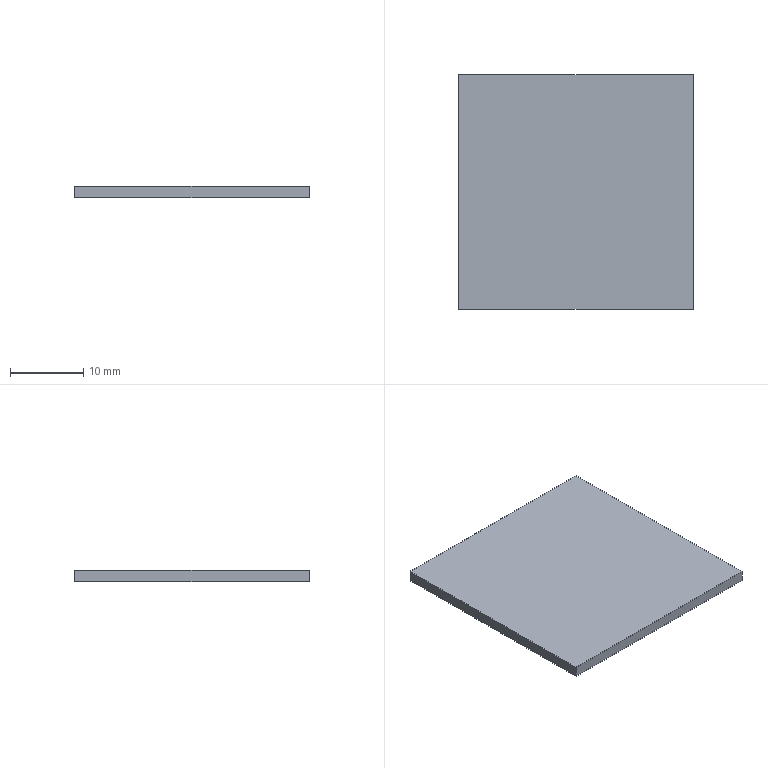Part | SolidWorks | features Extrusion 1 | 1 solid | 6 faces | box 32 x 32 x 1.5 mm | volume 1536 mm3 | plane 6
STEP:
#1=CARTESIAN_POINT('',(16.,-16.,0.));
#2=VERTEX_POINT('',#1);
#3=CARTESIAN_POINT('',(16.,16.,0.));
#4=VERTEX_POINT('',#3);
#5=CARTESIAN_POINT('',(16.,16.,0.));
#6=DIRECTION('',(0.,1.,0.));
#7=VECTOR('',#6,1000.);
#8=LINE('',#5,#7);
#9=EDGE_CURVE('',#2,#4,#8,.T.);
#10=ORIENTED_EDGE('',*,*,#9,.T.);
#11=CARTESIAN_POINT('',(16.,16.,1.5));
#12=VERTEX_POINT('',#11);
#13=CARTESIAN_POINT('',(16.,16.,1.5));
#14=DIRECTION('',(0.,0.,-1.));
#15=VECTOR('',#14,1000.);
#16=LINE('',#13,#15);
#17=EDGE_CURVE('',#12,#4,#16,.T.);
#18=ORIENTED_EDGE('',*,*,#17,.F.);
#19=CARTESIAN_POINT('',(16.,-16.,1.5));
#20=VERTEX_POINT('',#19);
#21=CARTESIAN_POINT('',(16.,16.,1.5));
#22=DIRECTION('',(0.,1.,0.));
#23=VECTOR('',#22,1000.);
#24=LINE('',#21,#23);
#25=EDGE_CURVE('',#20,#12,#24,.T.);
#26=ORIENTED_EDGE('',*,*,#25,.F.);
#27=CARTESIAN_POINT('',(16.,-16.,1.5));
#28=DIRECTION('',(0.,0.,-1.));
#29=VECTOR('',#28,1000.);
#30=LINE('',#27,#29);
#31=EDGE_CURVE('',#20,#2,#30,.T.);
#32=ORIENTED_EDGE('',*,*,#31,.T.);
#33=EDGE_LOOP('',(#10,#18,#26,#32));
#34=FACE_OUTER_BOUND('',#33,.T.);
#35=CARTESIAN_POINT('',(16.,16.,1.5));
#36=DIRECTION('',(-1.,0.,0.));
#37=DIRECTION('',(0.,-1.,0.));
#38=AXIS2_PLACEMENT_3D('',#35,#36,#37);
#39=PLANE('',#38);
#40=ADVANCED_FACE('',(#34),#39,.F.);
#41=CARTESIAN_POINT('',(-16.,16.,0.));
#42=VERTEX_POINT('',#41);
#43=CARTESIAN_POINT('',(-16.,16.,0.));
#44=DIRECTION('',(-1.,0.,0.));
#45=VECTOR('',#44,1000.);
#46=LINE('',#43,#45);
#47=EDGE_CURVE('',#4,#42,#46,.T.);
#48=ORIENTED_EDGE('',*,*,#47,.T.);
#49=CARTESIAN_POINT('',(-16.,16.,1.5));
#50=VERTEX_POINT('',#49);
#51=CARTESIAN_POINT('',(-16.,16.,1.5));
#52=DIRECTION('',(0.,0.,-1.));
#53=VECTOR('',#52,1000.);
#54=LINE('',#51,#53);
#55=EDGE_CURVE('',#50,#42,#54,.T.);
#56=ORIENTED_EDGE('',*,*,#55,.F.);
#57=CARTESIAN_POINT('',(-16.,16.,1.5));
#58=DIRECTION('',(-1.,0.,0.));
#59=VECTOR('',#58,1000.);
#60=LINE('',#57,#59);
#61=EDGE_CURVE('',#12,#50,#60,.T.);
#62=ORIENTED_EDGE('',*,*,#61,.F.);
#63=ORIENTED_EDGE('',*,*,#17,.T.);
#64=EDGE_LOOP('',(#48,#56,#62,#63));
#65=FACE_OUTER_BOUND('',#64,.T.);
#66=CARTESIAN_POINT('',(-16.,16.,1.5));
#67=DIRECTION('',(0.,-1.,0.));
#68=DIRECTION('',(0.,0.,-1.));
#69=AXIS2_PLACEMENT_3D('',#66,#67,#68);
#70=PLANE('',#69);
#71=ADVANCED_FACE('',(#65),#70,.F.);
#72=CARTESIAN_POINT('',(-16.,-16.,0.));
#73=VERTEX_POINT('',#72);
#74=CARTESIAN_POINT('',(-16.,16.,0.));
#75=DIRECTION('',(0.,-1.,0.));
#76=VECTOR('',#75,1000.);
#77=LINE('',#74,#76);
#78=EDGE_CURVE('',#42,#73,#77,.T.);
#79=ORIENTED_EDGE('',*,*,#78,.T.);
#80=CARTESIAN_POINT('',(-16.,-16.,1.5));
#81=VERTEX_POINT('',#80);
#82=CARTESIAN_POINT('',(-16.,-16.,1.5));
#83=DIRECTION('',(0.,0.,-1.));
#84=VECTOR('',#83,1000.);
#85=LINE('',#82,#84);
#86=EDGE_CURVE('',#81,#73,#85,.T.);
#87=ORIENTED_EDGE('',*,*,#86,.F.);
#88=CARTESIAN_POINT('',(-16.,16.,1.5));
#89=DIRECTION('',(0.,-1.,0.));
#90=VECTOR('',#89,1000.);
#91=LINE('',#88,#90);
#92=EDGE_CURVE('',#50,#81,#91,.T.);
#93=ORIENTED_EDGE('',*,*,#92,.F.);
#94=ORIENTED_EDGE('',*,*,#55,.T.);
#95=EDGE_LOOP('',(#79,#87,#93,#94));
#96=FACE_OUTER_BOUND('',#95,.T.);
#97=CARTESIAN_POINT('',(-16.,16.,1.5));
#98=DIRECTION('',(1.,0.,0.));
#99=DIRECTION('',(0.,1.,0.));
#100=AXIS2_PLACEMENT_3D('',#97,#98,#99);
#101=PLANE('',#100);
#102=ADVANCED_FACE('',(#96),#101,.F.);
#103=CARTESIAN_POINT('',(-16.,-16.,0.));
#104=DIRECTION('',(1.,0.,0.));
#105=VECTOR('',#104,1000.);
#106=LINE('',#103,#105);
#107=EDGE_CURVE('',#73,#2,#106,.T.);
#108=ORIENTED_EDGE('',*,*,#107,.T.);
#109=ORIENTED_EDGE('',*,*,#31,.F.);
#110=CARTESIAN_POINT('',(-16.,-16.,1.5));
#111=DIRECTION('',(1.,0.,0.));
#112=VECTOR('',#111,1000.);
#113=LINE('',#110,#112);
#114=EDGE_CURVE('',#81,#20,#113,.T.);
#115=ORIENTED_EDGE('',*,*,#114,.F.);
#116=ORIENTED_EDGE('',*,*,#86,.T.);
#117=EDGE_LOOP('',(#108,#109,#115,#116));
#118=FACE_OUTER_BOUND('',#117,.T.);
#119=CARTESIAN_POINT('',(-16.,-16.,1.5));
#120=DIRECTION('',(0.,1.,0.));
#121=DIRECTION('',(0.,0.,1.));
#122=AXIS2_PLACEMENT_3D('',#119,#120,#121);
#123=PLANE('',#122);
#124=ADVANCED_FACE('',(#118),#123,.F.);
#125=ORIENTED_EDGE('',*,*,#25,.T.);
#126=ORIENTED_EDGE('',*,*,#61,.T.);
#127=ORIENTED_EDGE('',*,*,#92,.T.);
#128=ORIENTED_EDGE('',*,*,#114,.T.);
#129=EDGE_LOOP('',(#125,#126,#127,#128));
#130=FACE_OUTER_BOUND('',#129,.T.);
#131=CARTESIAN_POINT('',(0.,0.,1.5));
#132=DIRECTION('',(0.,0.,1.));
#133=DIRECTION('',(1.,0.,0.));
#134=AXIS2_PLACEMENT_3D('',#131,#132,#133);
#135=PLANE('',#134);
#136=ADVANCED_FACE('',(#130),#135,.T.);
#137=ORIENTED_EDGE('',*,*,#9,.F.);
#138=ORIENTED_EDGE('',*,*,#107,.F.);
#139=ORIENTED_EDGE('',*,*,#78,.F.);
#140=ORIENTED_EDGE('',*,*,#47,.F.);
#141=EDGE_LOOP('',(#137,#138,#139,#140));
#142=FACE_OUTER_BOUND('',#141,.T.);
#143=CARTESIAN_POINT('',(0.,0.,0.));
#144=DIRECTION('',(0.,0.,1.));
#145=DIRECTION('',(1.,0.,0.));
#146=AXIS2_PLACEMENT_3D('',#143,#144,#145);
#147=PLANE('',#146);
#148=ADVANCED_FACE('',(#142),#147,.F.);
#149=CLOSED_SHELL('',(#40,#71,#102,#124,#136,#148));
#150=MANIFOLD_SOLID_BREP('',#149);
#151=CARTESIAN_POINT('',(0.,0.,0.));
#152=DIRECTION('',(0.,0.,1.));
#153=DIRECTION('',(1.,0.,0.));
#154=AXIS2_PLACEMENT_3D('',#151,#152,#153);
#155=(LENGTH_UNIT()NAMED_UNIT(*)SI_UNIT(.MILLI.,.METRE.));
#156=UNCERTAINTY_MEASURE_WITH_UNIT(LENGTH_MEASURE(0.00001),#155,'','');
#157=(NAMED_UNIT(*)PLANE_ANGLE_UNIT()SI_UNIT($,.RADIAN.));
#158=(NAMED_UNIT(*)SI_UNIT($,.STERADIAN.)SOLID_ANGLE_UNIT());
#159=(GEOMETRIC_REPRESENTATION_CONTEXT(3)GLOBAL_UNCERTAINTY_ASSIGNED_CONTEXT((#156))GLOBAL_UNIT_ASSIGNED_CONTEXT((#155,#157,#158))REPRESENTATION_CONTEXT('',''));
#160=ADVANCED_BREP_SHAPE_REPRESENTATION('',(#150,#154),#159);